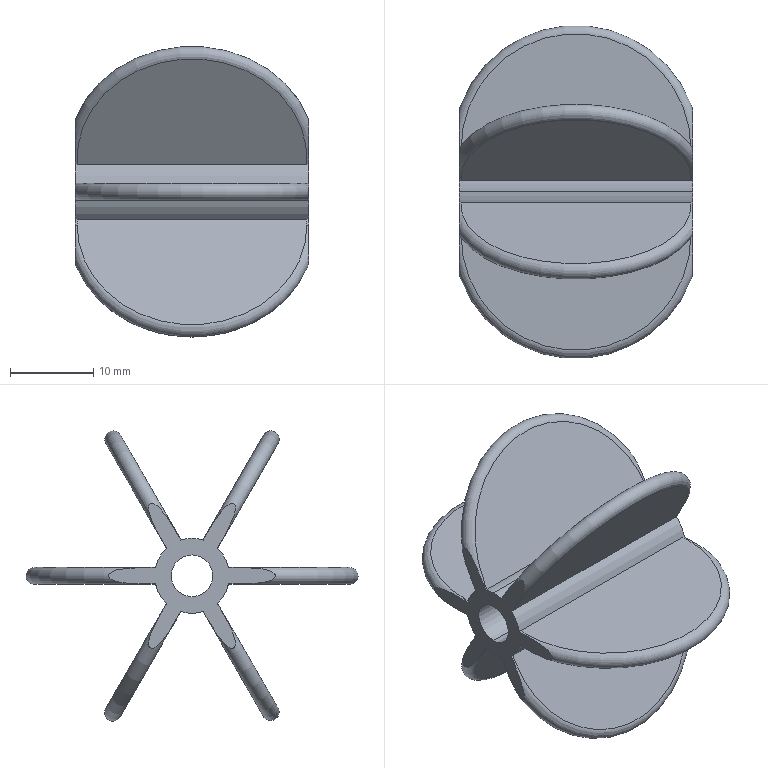Part | SolidWorks | features BaseBody 1 | 1 solid | 46 faces | box 28 x 40 x 34.909 mm | volume 5449 mm3 | torus 23 | plane 14 | cylinder 9 | commonest cylinder face diameters 9 x7 5 x2